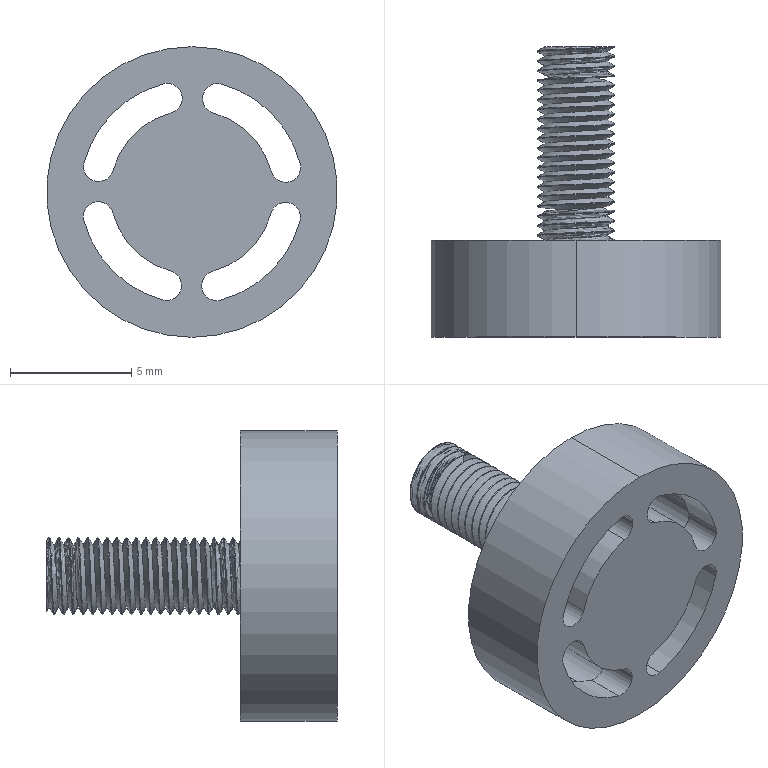Part | SolidWorks | features ICE 3, Extrusion 1, Helix 1, Scale 1, SweepCut 1 | 1 solid | 92 faces | box 12 x 12 x 12 mm | volume 351.083 mm3 | cylinder 83 | plane 7 | spline 2 | commonest cylinder face diameters 3.2 x41 1.24 x12 2.04 x12 5.96 x4 6.76 x4 9.24 x4